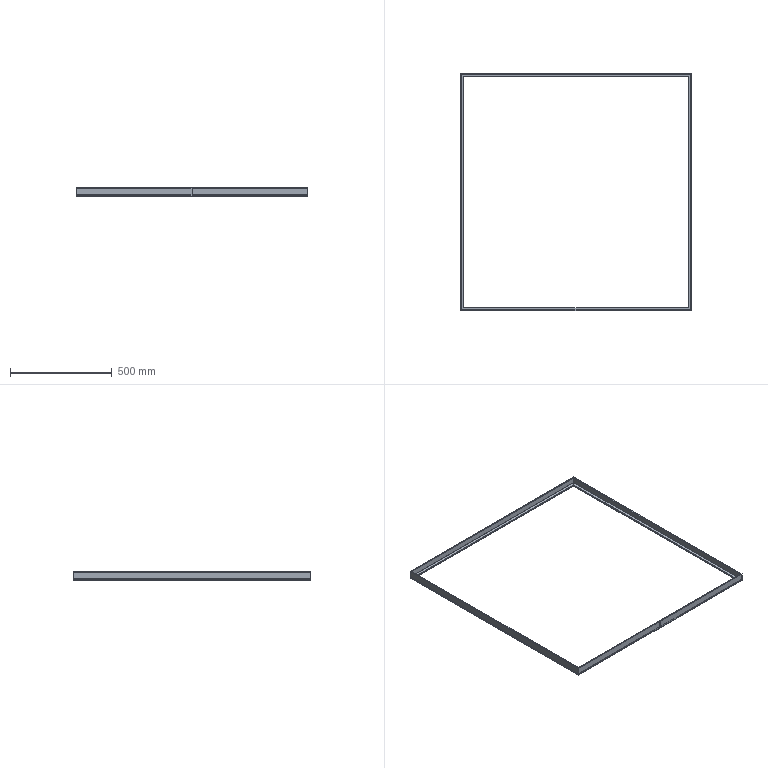Part | 1 solid | 90 faces | box 1140 x 1170 x 40 mm | volume 418841 mm3 | plane 90